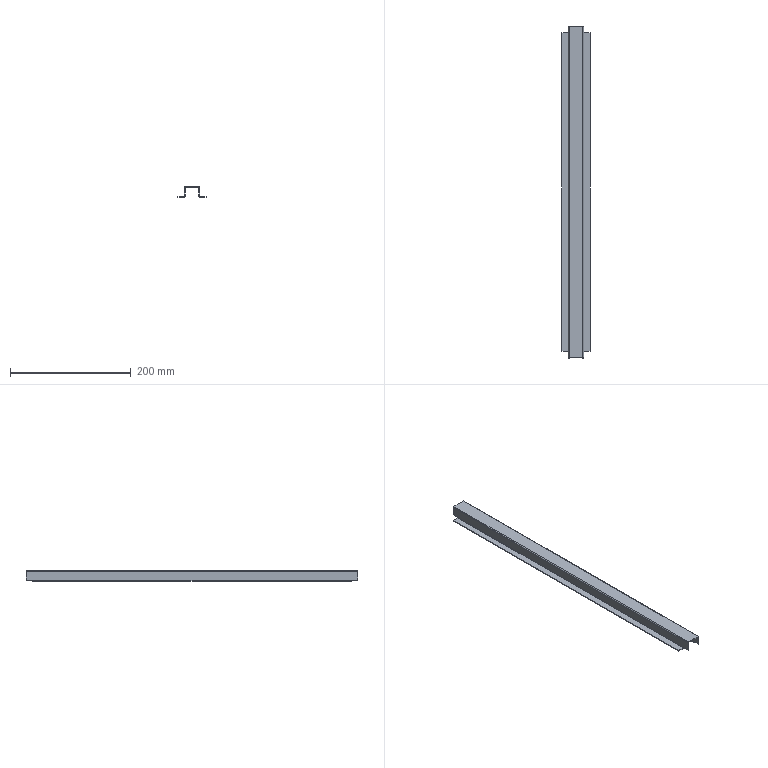Part | SolidWorks | features EdgeFlange 3, FlatPattern 1, ICE 1, SMBaseFlange 1, SheetMetal 1 | 1 solid | 46 faces | box 46.6 x 550 x 18 mm | volume 51368 mm3 | plane 38 | cylinder 8 | commonest cylinder face diameters 0.4 x4 2.8 x4
STEP:
#1=CARTESIAN_POINT('',(24.665,538.707,-16.6));
#2=VERTEX_POINT('',#1);
#3=CARTESIAN_POINT('',(24.665,10.707,-16.6));
#4=VERTEX_POINT('',#3);
#5=CARTESIAN_POINT('',(24.665,538.707,-16.6));
#6=DIRECTION('',(0.,-1.,0.));
#7=VECTOR('',#6,1000.);
#8=LINE('',#5,#7);
#9=EDGE_CURVE('',#2,#4,#8,.T.);
#10=ORIENTED_EDGE('',*,*,#9,.F.);
#11=CARTESIAN_POINT('',(24.665,538.707,-16.));
#12=VERTEX_POINT('',#11);
#13=CARTESIAN_POINT('',(24.665,538.707,0.));
#14=DIRECTION('',(0.,0.,-1.));
#15=VECTOR('',#14,1000.);
#16=LINE('',#13,#15);
#17=EDGE_CURVE('',#12,#2,#16,.T.);
#18=ORIENTED_EDGE('',*,*,#17,.F.);
#19=CARTESIAN_POINT('',(24.665,549.707,-16.));
#20=VERTEX_POINT('',#19);
#21=CARTESIAN_POINT('',(24.665,0.,-16.));
#22=DIRECTION('',(0.,-1.,0.));
#23=VECTOR('',#22,1000.);
#24=LINE('',#21,#23);
#25=EDGE_CURVE('',#20,#12,#24,.T.);
#26=ORIENTED_EDGE('',*,*,#25,.F.);
#27=CARTESIAN_POINT('',(24.665,549.707,-1.4));
#28=VERTEX_POINT('',#27);
#29=CARTESIAN_POINT('',(24.665,549.707,-18.));
#30=DIRECTION('',(0.,0.,-1.));
#31=VECTOR('',#30,1000.);
#32=LINE('',#29,#31);
#33=EDGE_CURVE('',#28,#20,#32,.T.);
#34=ORIENTED_EDGE('',*,*,#33,.F.);
#35=CARTESIAN_POINT('',(24.665,-0.2928,-1.4));
#36=VERTEX_POINT('',#35);
#37=CARTESIAN_POINT('',(24.665,0.,-1.4));
#38=DIRECTION('',(0.,-1.,0.));
#39=VECTOR('',#38,1000.);
#40=LINE('',#37,#39);
#41=EDGE_CURVE('',#28,#36,#40,.T.);
#42=ORIENTED_EDGE('',*,*,#41,.T.);
#43=CARTESIAN_POINT('',(24.665,-0.2928,-16.));
#44=VERTEX_POINT('',#43);
#45=CARTESIAN_POINT('',(24.665,-0.2928,-1.2));
#46=DIRECTION('',(0.,0.,1.));
#47=VECTOR('',#46,1000.);
#48=LINE('',#45,#47);
#49=EDGE_CURVE('',#44,#36,#48,.T.);
#50=ORIENTED_EDGE('',*,*,#49,.F.);
#51=CARTESIAN_POINT('',(24.665,10.707,-16.));
#52=VERTEX_POINT('',#51);
#53=CARTESIAN_POINT('',(24.665,0.,-16.));
#54=DIRECTION('',(0.,-1.,0.));
#55=VECTOR('',#54,1000.);
#56=LINE('',#53,#55);
#57=EDGE_CURVE('',#52,#44,#56,.T.);
#58=ORIENTED_EDGE('',*,*,#57,.F.);
#59=CARTESIAN_POINT('',(24.665,10.707,0.));
#60=DIRECTION('',(0.,0.,1.));
#61=VECTOR('',#60,1000.);
#62=LINE('',#59,#61);
#63=EDGE_CURVE('',#4,#52,#62,.T.);
#64=ORIENTED_EDGE('',*,*,#63,.F.);
#65=EDGE_LOOP('',(#10,#18,#26,#34,#42,#50,#58,#64));
#66=FACE_OUTER_BOUND('',#65,.T.);
#67=CARTESIAN_POINT('',(24.665,0.,0.));
#68=DIRECTION('',(1.,0.,0.));
#69=DIRECTION('',(0.,0.,-1.));
#70=AXIS2_PLACEMENT_3D('',#67,#68,#69);
#71=PLANE('',#70);
#72=ADVANCED_FACE('',(#66),#71,.T.);
#73=CARTESIAN_POINT('',(23.465,538.707,-16.));
#74=VERTEX_POINT('',#73);
#75=CARTESIAN_POINT('',(23.465,538.707,-16.6));
#76=VERTEX_POINT('',#75);
#77=CARTESIAN_POINT('',(23.465,538.707,0.));
#78=DIRECTION('',(0.,0.,-1.));
#79=VECTOR('',#78,1000.);
#80=LINE('',#77,#79);
#81=EDGE_CURVE('',#74,#76,#80,.T.);
#82=ORIENTED_EDGE('',*,*,#81,.T.);
#83=CARTESIAN_POINT('',(23.465,10.707,-16.6));
#84=VERTEX_POINT('',#83);
#85=CARTESIAN_POINT('',(23.465,538.707,-16.6));
#86=DIRECTION('',(0.,-1.,0.));
#87=VECTOR('',#86,1000.);
#88=LINE('',#85,#87);
#89=EDGE_CURVE('',#76,#84,#88,.T.);
#90=ORIENTED_EDGE('',*,*,#89,.T.);
#91=CARTESIAN_POINT('',(23.465,10.707,-16.));
#92=VERTEX_POINT('',#91);
#93=CARTESIAN_POINT('',(23.465,10.707,0.));
#94=DIRECTION('',(0.,0.,1.));
#95=VECTOR('',#94,1000.);
#96=LINE('',#93,#95);
#97=EDGE_CURVE('',#84,#92,#96,.T.);
#98=ORIENTED_EDGE('',*,*,#97,.T.);
#99=CARTESIAN_POINT('',(23.465,-0.2928,-16.));
#100=VERTEX_POINT('',#99);
#101=CARTESIAN_POINT('',(23.465,0.,-16.));
#102=DIRECTION('',(0.,-1.,0.));
#103=VECTOR('',#102,1000.);
#104=LINE('',#101,#103);
#105=EDGE_CURVE('',#92,#100,#104,.T.);
#106=ORIENTED_EDGE('',*,*,#105,.T.);
#107=CARTESIAN_POINT('',(23.465,-0.2928,-1.4));
#108=VERTEX_POINT('',#107);
#109=CARTESIAN_POINT('',(23.465,-0.2928,0.));
#110=DIRECTION('',(0.,0.,1.));
#111=VECTOR('',#110,1000.);
#112=LINE('',#109,#111);
#113=EDGE_CURVE('',#100,#108,#112,.T.);
#114=ORIENTED_EDGE('',*,*,#113,.T.);
#115=CARTESIAN_POINT('',(23.465,549.707,-1.4));
#116=VERTEX_POINT('',#115);
#117=CARTESIAN_POINT('',(23.465,549.707,-1.4));
#118=DIRECTION('',(0.,-1.,0.));
#119=VECTOR('',#118,1000.);
#120=LINE('',#117,#119);
#121=EDGE_CURVE('',#116,#108,#120,.T.);
#122=ORIENTED_EDGE('',*,*,#121,.F.);
#123=CARTESIAN_POINT('',(23.465,549.707,-16.));
#124=VERTEX_POINT('',#123);
#125=CARTESIAN_POINT('',(23.465,549.707,0.));
#126=DIRECTION('',(0.,0.,-1.));
#127=VECTOR('',#126,1000.);
#128=LINE('',#125,#127);
#129=EDGE_CURVE('',#116,#124,#128,.T.);
#130=ORIENTED_EDGE('',*,*,#129,.T.);
#131=CARTESIAN_POINT('',(23.465,0.,-16.));
#132=DIRECTION('',(0.,-1.,0.));
#133=VECTOR('',#132,1000.);
#134=LINE('',#131,#133);
#135=EDGE_CURVE('',#124,#74,#134,.T.);
#136=ORIENTED_EDGE('',*,*,#135,.T.);
#137=EDGE_LOOP('',(#82,#90,#98,#106,#114,#122,#130,#136));
#138=FACE_OUTER_BOUND('',#137,.T.);
#139=CARTESIAN_POINT('',(23.465,0.,0.));
#140=DIRECTION('',(1.,0.,0.));
#141=DIRECTION('',(0.,0.,-1.));
#142=AXIS2_PLACEMENT_3D('',#139,#140,#141);
#143=PLANE('',#142);
#144=ADVANCED_FACE('',(#138),#143,.F.);
#145=ORIENTED_EDGE('',*,*,#33,.T.);
#146=CARTESIAN_POINT('',(23.465,549.707,-16.));
#147=DIRECTION('',(1.,0.,0.));
#148=VECTOR('',#147,1000.);
#149=LINE('',#146,#148);
#150=EDGE_CURVE('',#124,#20,#149,.T.);
#151=ORIENTED_EDGE('',*,*,#150,.F.);
#152=ORIENTED_EDGE('',*,*,#129,.F.);
#153=CARTESIAN_POINT('',(24.665,549.707,-1.4));
#154=DIRECTION('',(1.,0.,0.));
#155=VECTOR('',#154,1000.);
#156=LINE('',#153,#155);
#157=EDGE_CURVE('',#116,#28,#156,.T.);
#158=ORIENTED_EDGE('',*,*,#157,.T.);
#159=EDGE_LOOP('',(#145,#151,#152,#158));
#160=FACE_OUTER_BOUND('',#159,.T.);
#161=CARTESIAN_POINT('',(24.665,549.707,-18.));
#162=DIRECTION('',(0.,1.,0.));
#163=DIRECTION('',(0.,0.,1.));
#164=AXIS2_PLACEMENT_3D('',#161,#162,#163);
#165=PLANE('',#164);
#166=ADVANCED_FACE('',(#160),#165,.T.);
#167=CARTESIAN_POINT('',(-0.3354,10.707,-16.));
#168=VERTEX_POINT('',#167);
#169=CARTESIAN_POINT('',(-0.3354,-0.2928,-16.));
#170=VERTEX_POINT('',#169);
#171=CARTESIAN_POINT('',(-0.3354,0.,-16.));
#172=DIRECTION('',(0.,-1.,0.));
#173=VECTOR('',#172,1000.);
#174=LINE('',#171,#173);
#175=EDGE_CURVE('',#168,#170,#174,.T.);
#176=ORIENTED_EDGE('',*,*,#175,.T.);
#177=CARTESIAN_POINT('',(-0.3354,-0.2928,-1.4));
#178=VERTEX_POINT('',#177);
#179=CARTESIAN_POINT('',(-0.3354,-0.2928,-1.2));
#180=DIRECTION('',(0.,0.,-1.));
#181=VECTOR('',#180,1000.);
#182=LINE('',#179,#181);
#183=EDGE_CURVE('',#178,#170,#182,.T.);
#184=ORIENTED_EDGE('',*,*,#183,.F.);
#185=CARTESIAN_POINT('',(-0.3354,549.707,-1.4));
#186=VERTEX_POINT('',#185);
#187=CARTESIAN_POINT('',(-0.3354,-0.2928,-1.4));
#188=DIRECTION('',(0.,-1.,0.));
#189=VECTOR('',#188,1000.);
#190=LINE('',#187,#189);
#191=EDGE_CURVE('',#186,#178,#190,.T.);
#192=ORIENTED_EDGE('',*,*,#191,.F.);
#193=CARTESIAN_POINT('',(-0.3354,549.707,-16.));
#194=VERTEX_POINT('',#193);
#195=CARTESIAN_POINT('',(-0.3354,549.707,-18.));
#196=DIRECTION('',(0.,0.,1.));
#197=VECTOR('',#196,1000.);
#198=LINE('',#195,#197);
#199=EDGE_CURVE('',#194,#186,#198,.T.);
#200=ORIENTED_EDGE('',*,*,#199,.F.);
#201=CARTESIAN_POINT('',(-0.3354,538.707,-16.));
#202=VERTEX_POINT('',#201);
#203=CARTESIAN_POINT('',(-0.3354,0.,-16.));
#204=DIRECTION('',(0.,-1.,0.));
#205=VECTOR('',#204,1000.);
#206=LINE('',#203,#205);
#207=EDGE_CURVE('',#194,#202,#206,.T.);
#208=ORIENTED_EDGE('',*,*,#207,.T.);
#209=CARTESIAN_POINT('',(-0.3354,538.707,-16.6));
#210=VERTEX_POINT('',#209);
#211=CARTESIAN_POINT('',(-0.3354,538.707,0.));
#212=DIRECTION('',(0.,0.,-1.));
#213=VECTOR('',#212,1000.);
#214=LINE('',#211,#213);
#215=EDGE_CURVE('',#202,#210,#214,.T.);
#216=ORIENTED_EDGE('',*,*,#215,.T.);
#217=CARTESIAN_POINT('',(-0.3354,10.707,-16.6));
#218=VERTEX_POINT('',#217);
#219=CARTESIAN_POINT('',(-0.3354,10.707,-16.6));
#220=DIRECTION('',(0.,1.,0.));
#221=VECTOR('',#220,1000.);
#222=LINE('',#219,#221);
#223=EDGE_CURVE('',#218,#210,#222,.T.);
#224=ORIENTED_EDGE('',*,*,#223,.F.);
#225=CARTESIAN_POINT('',(-0.3354,10.707,0.));
#226=DIRECTION('',(0.,0.,1.));
#227=VECTOR('',#226,1000.);
#228=LINE('',#225,#227);
#229=EDGE_CURVE('',#218,#168,#228,.T.);
#230=ORIENTED_EDGE('',*,*,#229,.T.);
#231=EDGE_LOOP('',(#176,#184,#192,#200,#208,#216,#224,#230));
#232=FACE_OUTER_BOUND('',#231,.T.);
#233=CARTESIAN_POINT('',(-0.3354,0.,0.));
#234=DIRECTION('',(1.,0.,0.));
#235=DIRECTION('',(0.,0.,-1.));
#236=AXIS2_PLACEMENT_3D('',#233,#234,#235);
#237=PLANE('',#236);
#238=ADVANCED_FACE('',(#232),#237,.F.);
#239=CARTESIAN_POINT('',(0.8646,-0.2928,-1.4));
#240=VERTEX_POINT('',#239);
#241=CARTESIAN_POINT('',(0.8646,-0.2928,-16.));
#242=VERTEX_POINT('',#241);
#243=CARTESIAN_POINT('',(0.8646,-0.2928,0.));
#244=DIRECTION('',(0.,0.,-1.));
#245=VECTOR('',#244,1000.);
#246=LINE('',#243,#245);
#247=EDGE_CURVE('',#240,#242,#246,.T.);
#248=ORIENTED_EDGE('',*,*,#247,.T.);
#249=CARTESIAN_POINT('',(0.8646,10.707,-16.));
#250=VERTEX_POINT('',#249);
#251=CARTESIAN_POINT('',(0.8646,0.,-16.));
#252=DIRECTION('',(0.,-1.,0.));
#253=VECTOR('',#252,1000.);
#254=LINE('',#251,#253);
#255=EDGE_CURVE('',#250,#242,#254,.T.);
#256=ORIENTED_EDGE('',*,*,#255,.F.);
#257=CARTESIAN_POINT('',(0.8646,10.707,-16.6));
#258=VERTEX_POINT('',#257);
#259=CARTESIAN_POINT('',(0.8646,10.707,0.));
#260=DIRECTION('',(0.,0.,1.));
#261=VECTOR('',#260,1000.);
#262=LINE('',#259,#261);
#263=EDGE_CURVE('',#258,#250,#262,.T.);
#264=ORIENTED_EDGE('',*,*,#263,.F.);
#265=CARTESIAN_POINT('',(0.8646,538.707,-16.6));
#266=VERTEX_POINT('',#265);
#267=CARTESIAN_POINT('',(0.8646,10.707,-16.6));
#268=DIRECTION('',(0.,1.,0.));
#269=VECTOR('',#268,1000.);
#270=LINE('',#267,#269);
#271=EDGE_CURVE('',#258,#266,#270,.T.);
#272=ORIENTED_EDGE('',*,*,#271,.T.);
#273=CARTESIAN_POINT('',(0.8646,538.707,-16.));
#274=VERTEX_POINT('',#273);
#275=CARTESIAN_POINT('',(0.8646,538.707,0.));
#276=DIRECTION('',(0.,0.,-1.));
#277=VECTOR('',#276,1000.);
#278=LINE('',#275,#277);
#279=EDGE_CURVE('',#274,#266,#278,.T.);
#280=ORIENTED_EDGE('',*,*,#279,.F.);
#281=CARTESIAN_POINT('',(0.8646,549.707,-16.));
#282=VERTEX_POINT('',#281);
#283=CARTESIAN_POINT('',(0.8646,0.,-16.));
#284=DIRECTION('',(0.,-1.,0.));
#285=VECTOR('',#284,1000.);
#286=LINE('',#283,#285);
#287=EDGE_CURVE('',#282,#274,#286,.T.);
#288=ORIENTED_EDGE('',*,*,#287,.F.);
#289=CARTESIAN_POINT('',(0.8646,549.707,-1.4));
#290=VERTEX_POINT('',#289);
#291=CARTESIAN_POINT('',(0.8646,549.707,0.));
#292=DIRECTION('',(0.,0.,1.));
#293=VECTOR('',#292,1000.);
#294=LINE('',#291,#293);
#295=EDGE_CURVE('',#282,#290,#294,.T.);
#296=ORIENTED_EDGE('',*,*,#295,.T.);
#297=CARTESIAN_POINT('',(0.8646,-0.2928,-1.4));
#298=DIRECTION('',(0.,1.,0.));
#299=VECTOR('',#298,1000.);
#300=LINE('',#297,#299);
#301=EDGE_CURVE('',#240,#290,#300,.T.);
#302=ORIENTED_EDGE('',*,*,#301,.F.);
#303=EDGE_LOOP('',(#248,#256,#264,#272,#280,#288,#296,#302));
#304=FACE_OUTER_BOUND('',#303,.T.);
#305=CARTESIAN_POINT('',(0.8646,0.,0.));
#306=DIRECTION('',(1.,0.,0.));
#307=DIRECTION('',(0.,0.,-1.));
#308=AXIS2_PLACEMENT_3D('',#305,#306,#307);
#309=PLANE('',#308);
#310=ADVANCED_FACE('',(#304),#309,.T.);
#311=ORIENTED_EDGE('',*,*,#183,.T.);
#312=CARTESIAN_POINT('',(-0.3354,-0.2928,-16.));
#313=DIRECTION('',(1.,0.,0.));
#314=VECTOR('',#313,1000.);
#315=LINE('',#312,#314);
#316=EDGE_CURVE('',#170,#242,#315,.T.);
#317=ORIENTED_EDGE('',*,*,#316,.T.);
#318=ORIENTED_EDGE('',*,*,#247,.F.);
#319=CARTESIAN_POINT('',(-0.3354,-0.2928,-1.4));
#320=DIRECTION('',(-1.,0.,0.));
#321=VECTOR('',#320,1000.);
#322=LINE('',#319,#321);
#323=EDGE_CURVE('',#240,#178,#322,.T.);
#324=ORIENTED_EDGE('',*,*,#323,.T.);
#325=EDGE_LOOP('',(#311,#317,#318,#324));
#326=FACE_OUTER_BOUND('',#325,.T.);
#327=CARTESIAN_POINT('',(-0.3354,-0.2928,-1.2));
#328=DIRECTION('',(0.,-1.,0.));
#329=DIRECTION('',(0.,0.,-1.));
#330=AXIS2_PLACEMENT_3D('',#327,#328,#329);
#331=PLANE('',#330);
#332=ADVANCED_FACE('',(#326),#331,.T.);
#333=ORIENTED_EDGE('',*,*,#295,.F.);
#334=CARTESIAN_POINT('',(-0.3354,549.707,-16.));
#335=DIRECTION('',(1.,0.,0.));
#336=VECTOR('',#335,1000.);
#337=LINE('',#334,#336);
#338=EDGE_CURVE('',#194,#282,#337,.T.);
#339=ORIENTED_EDGE('',*,*,#338,.F.);
#340=ORIENTED_EDGE('',*,*,#199,.T.);
#341=CARTESIAN_POINT('',(0.8646,549.707,-1.4));
#342=DIRECTION('',(-1.,0.,0.));
#343=VECTOR('',#342,1000.);
#344=LINE('',#341,#343);
#345=EDGE_CURVE('',#290,#186,#344,.T.);
#346=ORIENTED_EDGE('',*,*,#345,.F.);
#347=EDGE_LOOP('',(#333,#339,#340,#346));
#348=FACE_OUTER_BOUND('',#347,.T.);
#349=CARTESIAN_POINT('',(-0.3354,549.707,-18.));
#350=DIRECTION('',(0.,1.,0.));
#351=DIRECTION('',(0.,0.,1.));
#352=AXIS2_PLACEMENT_3D('',#349,#350,#351);
#353=PLANE('',#352);
#354=ADVANCED_FACE('',(#348),#353,.T.);
#355=ORIENTED_EDGE('',*,*,#113,.F.);
#356=CARTESIAN_POINT('',(23.465,-0.2928,-16.));
#357=DIRECTION('',(1.,0.,0.));
#358=VECTOR('',#357,1000.);
#359=LINE('',#356,#358);
#360=EDGE_CURVE('',#100,#44,#359,.T.);
#361=ORIENTED_EDGE('',*,*,#360,.T.);
#362=ORIENTED_EDGE('',*,*,#49,.T.);
#363=CARTESIAN_POINT('',(23.465,-0.2928,-1.4));
#364=DIRECTION('',(1.,0.,0.));
#365=VECTOR('',#364,1000.);
#366=LINE('',#363,#365);
#367=EDGE_CURVE('',#108,#36,#366,.T.);
#368=ORIENTED_EDGE('',*,*,#367,.F.);
#369=EDGE_LOOP('',(#355,#361,#362,#368));
#370=FACE_OUTER_BOUND('',#369,.T.);
#371=CARTESIAN_POINT('',(24.665,-0.2928,-1.2));
#372=DIRECTION('',(0.,-1.,0.));
#373=DIRECTION('',(0.,0.,-1.));
#374=AXIS2_PLACEMENT_3D('',#371,#372,#373);
#375=PLANE('',#374);
#376=ADVANCED_FACE('',(#370),#375,.T.);
#377=CARTESIAN_POINT('',(1.065,-0.2928,-1.2));
#378=VERTEX_POINT('',#377);
#379=CARTESIAN_POINT('',(23.265,-0.2928,-1.2));
#380=VERTEX_POINT('',#379);
#381=CARTESIAN_POINT('',(-0.3354,-0.2928,-1.2));
#382=DIRECTION('',(1.,0.,0.));
#383=VECTOR('',#382,1000.);
#384=LINE('',#381,#383);
#385=EDGE_CURVE('',#378,#380,#384,.T.);
#386=ORIENTED_EDGE('',*,*,#385,.F.);
#387=CARTESIAN_POINT('',(1.065,549.707,-1.2));
#388=VERTEX_POINT('',#387);
#389=CARTESIAN_POINT('',(1.065,549.707,-1.2));
#390=DIRECTION('',(0.,-1.,0.));
#391=VECTOR('',#390,1000.);
#392=LINE('',#389,#391);
#393=EDGE_CURVE('',#388,#378,#392,.T.);
#394=ORIENTED_EDGE('',*,*,#393,.F.);
#395=CARTESIAN_POINT('',(23.265,549.707,-1.2));
#396=VERTEX_POINT('',#395);
#397=CARTESIAN_POINT('',(-0.3354,549.707,-1.2));
#398=DIRECTION('',(-1.,0.,0.));
#399=VECTOR('',#398,1000.);
#400=LINE('',#397,#399);
#401=EDGE_CURVE('',#396,#388,#400,.T.);
#402=ORIENTED_EDGE('',*,*,#401,.F.);
#403=CARTESIAN_POINT('',(23.265,-0.2928,-1.2));
#404=DIRECTION('',(0.,1.,0.));
#405=VECTOR('',#404,1000.);
#406=LINE('',#403,#405);
#407=EDGE_CURVE('',#380,#396,#406,.T.);
#408=ORIENTED_EDGE('',*,*,#407,.F.);
#409=EDGE_LOOP('',(#386,#394,#402,#408));
#410=FACE_OUTER_BOUND('',#409,.T.);
#411=CARTESIAN_POINT('',(0.,0.,-1.2));
#412=DIRECTION('',(0.,0.,-1.));
#413=DIRECTION('',(-1.,0.,0.));
#414=AXIS2_PLACEMENT_3D('',#411,#412,#413);
#415=PLANE('',#414);
#416=ADVANCED_FACE('',(#410),#415,.T.);
#417=CARTESIAN_POINT('',(1.065,549.707,0.));
#418=VERTEX_POINT('',#417);
#419=CARTESIAN_POINT('',(1.065,-0.2928,0.));
#420=VERTEX_POINT('',#419);
#421=CARTESIAN_POINT('',(1.065,549.707,0.));
#422=DIRECTION('',(0.,-1.,0.));
#423=VECTOR('',#422,1000.);
#424=LINE('',#421,#423);
#425=EDGE_CURVE('',#418,#420,#424,.T.);
#426=ORIENTED_EDGE('',*,*,#425,.T.);
#427=CARTESIAN_POINT('',(23.265,-0.2928,0.));
#428=VERTEX_POINT('',#427);
#429=CARTESIAN_POINT('',(-0.3354,-0.2928,0.));
#430=DIRECTION('',(1.,0.,0.));
#431=VECTOR('',#430,1000.);
#432=LINE('',#429,#431);
#433=EDGE_CURVE('',#420,#428,#432,.T.);
#434=ORIENTED_EDGE('',*,*,#433,.T.);
#435=CARTESIAN_POINT('',(23.265,549.707,0.));
#436=VERTEX_POINT('',#435);
#437=CARTESIAN_POINT('',(23.265,-0.2928,0.));
#438=DIRECTION('',(0.,1.,0.));
#439=VECTOR('',#438,1000.);
#440=LINE('',#437,#439);
#441=EDGE_CURVE('',#428,#436,#440,.T.);
#442=ORIENTED_EDGE('',*,*,#441,.T.);
#443=CARTESIAN_POINT('',(-0.3354,549.707,0.));
#444=DIRECTION('',(-1.,0.,0.));
#445=VECTOR('',#444,1000.);
#446=LINE('',#443,#445);
#447=EDGE_CURVE('',#436,#418,#446,.T.);
#448=ORIENTED_EDGE('',*,*,#447,.T.);
#449=EDGE_LOOP('',(#426,#434,#442,#448));
#450=FACE_OUTER_BOUND('',#449,.T.);
#451=CARTESIAN_POINT('',(0.,0.,0.));
#452=DIRECTION('',(0.,0.,-1.));
#453=DIRECTION('',(-1.,0.,0.));
#454=AXIS2_PLACEMENT_3D('',#451,#452,#453);
#455=PLANE('',#454);
#456=ADVANCED_FACE('',(#450),#455,.F.);
#457=ORIENTED_EDGE('',*,*,#401,.T.);
#458=CARTESIAN_POINT('',(1.065,549.707,-1.2));
#459=DIRECTION('',(0.,0.,1.));
#460=VECTOR('',#459,1000.);
#461=LINE('',#458,#460);
#462=EDGE_CURVE('',#388,#418,#461,.T.);
#463=ORIENTED_EDGE('',*,*,#462,.T.);
#464=ORIENTED_EDGE('',*,*,#447,.F.);
#465=CARTESIAN_POINT('',(23.265,549.707,-1.2));
#466=DIRECTION('',(0.,0.,1.));
#467=VECTOR('',#466,1000.);
#468=LINE('',#465,#467);
#469=EDGE_CURVE('',#396,#436,#468,.T.);
#470=ORIENTED_EDGE('',*,*,#469,.F.);
#471=EDGE_LOOP('',(#457,#463,#464,#470));
#472=FACE_OUTER_BOUND('',#471,.T.);
#473=CARTESIAN_POINT('',(-0.3354,549.707,-1.2));
#474=DIRECTION('',(0.,1.,0.));
#475=DIRECTION('',(0.,0.,1.));
#476=AXIS2_PLACEMENT_3D('',#473,#474,#475);
#477=PLANE('',#476);
#478=ADVANCED_FACE('',(#472),#477,.T.);
#479=CARTESIAN_POINT('',(1.065,-0.2928,-1.2));
#480=DIRECTION('',(0.,0.,1.));
#481=VECTOR('',#480,1000.);
#482=LINE('',#479,#481);
#483=EDGE_CURVE('',#378,#420,#482,.T.);
#484=ORIENTED_EDGE('',*,*,#483,.F.);
#485=ORIENTED_EDGE('',*,*,#385,.T.);
#486=CARTESIAN_POINT('',(23.265,-0.2928,-1.2));
#487=DIRECTION('',(0.,0.,1.));
#488=VECTOR('',#487,1000.);
#489=LINE('',#486,#488);
#490=EDGE_CURVE('',#380,#428,#489,.T.);
#491=ORIENTED_EDGE('',*,*,#490,.T.);
#492=ORIENTED_EDGE('',*,*,#433,.F.);
#493=EDGE_LOOP('',(#484,#485,#491,#492));
#494=FACE_OUTER_BOUND('',#493,.T.);
#495=CARTESIAN_POINT('',(-0.3354,-0.2928,-1.2));
#496=DIRECTION('',(0.,-1.,0.));
#497=DIRECTION('',(0.,0.,-1.));
#498=AXIS2_PLACEMENT_3D('',#495,#496,#497);
#499=PLANE('',#498);
#500=ADVANCED_FACE('',(#494),#499,.T.);
#501=ORIENTED_EDGE('',*,*,#157,.F.);
#502=CARTESIAN_POINT('',(23.265,549.707,-1.4));
#503=DIRECTION('',(0.,1.,0.));
#504=DIRECTION('',(0.,0.,-1.));
#505=AXIS2_PLACEMENT_3D('',#502,#503,#504);
#506=CIRCLE('',#505,0.2);
#507=EDGE_CURVE('',#396,#116,#506,.T.);
#508=ORIENTED_EDGE('',*,*,#507,.F.);
#509=ORIENTED_EDGE('',*,*,#469,.T.);
#510=CARTESIAN_POINT('',(23.265,549.707,-1.4));
#511=DIRECTION('',(0.,1.,0.));
#512=DIRECTION('',(0.,0.,-1.));
#513=AXIS2_PLACEMENT_3D('',#510,#511,#512);
#514=CIRCLE('',#513,1.4);
#515=EDGE_CURVE('',#436,#28,#514,.T.);
#516=ORIENTED_EDGE('',*,*,#515,.T.);
#517=EDGE_LOOP('',(#501,#508,#509,#516));
#518=FACE_OUTER_BOUND('',#517,.T.);
#519=CARTESIAN_POINT('',(23.265,549.707,-1.4));
#520=DIRECTION('',(0.,1.,0.));
#521=DIRECTION('',(0.,0.,1.));
#522=AXIS2_PLACEMENT_3D('',#519,#520,#521);
#523=PLANE('',#522);
#524=ADVANCED_FACE('',(#518),#523,.T.);
#525=CARTESIAN_POINT('',(23.265,-0.2928,-1.4));
#526=DIRECTION('',(0.,-1.,0.));
#527=DIRECTION('',(0.,0.,-1.));
#528=AXIS2_PLACEMENT_3D('',#525,#526,#527);
#529=CIRCLE('',#528,0.2);
#530=EDGE_CURVE('',#108,#380,#529,.T.);
#531=ORIENTED_EDGE('',*,*,#530,.F.);
#532=ORIENTED_EDGE('',*,*,#367,.T.);
#533=CARTESIAN_POINT('',(23.265,-0.2928,-1.4));
#534=DIRECTION('',(0.,-1.,0.));
#535=DIRECTION('',(0.,0.,-1.));
#536=AXIS2_PLACEMENT_3D('',#533,#534,#535);
#537=CIRCLE('',#536,1.4);
#538=EDGE_CURVE('',#36,#428,#537,.T.);
#539=ORIENTED_EDGE('',*,*,#538,.T.);
#540=ORIENTED_EDGE('',*,*,#490,.F.);
#541=EDGE_LOOP('',(#531,#532,#539,#540));
#542=FACE_OUTER_BOUND('',#541,.T.);
#543=CARTESIAN_POINT('',(23.265,-0.2928,-1.4));
#544=DIRECTION('',(0.,1.,0.));
#545=DIRECTION('',(0.,0.,1.));
#546=AXIS2_PLACEMENT_3D('',#543,#544,#545);
#547=PLANE('',#546);
#548=ADVANCED_FACE('',(#542),#547,.F.);
#549=ORIENTED_EDGE('',*,*,#441,.F.);
#550=ORIENTED_EDGE('',*,*,#538,.F.);
#551=ORIENTED_EDGE('',*,*,#41,.F.);
#552=ORIENTED_EDGE('',*,*,#515,.F.);
#553=EDGE_LOOP('',(#549,#550,#551,#552));
#554=FACE_OUTER_BOUND('',#553,.T.);
#555=CARTESIAN_POINT('',(23.265,-0.2928,-1.4));
#556=DIRECTION('',(0.,-1.,0.));
#557=DIRECTION('',(1.,0.,0.));
#558=AXIS2_PLACEMENT_3D('',#555,#556,#557);
#559=CYLINDRICAL_SURFACE('',#558,1.4);
#560=ADVANCED_FACE('',(#554),#559,.T.);
#561=ORIENTED_EDGE('',*,*,#407,.T.);
#562=ORIENTED_EDGE('',*,*,#507,.T.);
#563=ORIENTED_EDGE('',*,*,#121,.T.);
#564=ORIENTED_EDGE('',*,*,#530,.T.);
#565=EDGE_LOOP('',(#561,#562,#563,#564));
#566=FACE_OUTER_BOUND('',#565,.T.);
#567=CARTESIAN_POINT('',(23.265,-0.2928,-1.4));
#568=DIRECTION('',(0.,-1.,0.));
#569=DIRECTION('',(1.,0.,0.));
#570=AXIS2_PLACEMENT_3D('',#567,#568,#569);
#571=CYLINDRICAL_SURFACE('',#570,0.2);
#572=ADVANCED_FACE('',(#566),#571,.F.);
#573=ORIENTED_EDGE('',*,*,#323,.F.);
#574=CARTESIAN_POINT('',(1.065,-0.2928,-1.4));
#575=DIRECTION('',(0.,-1.,0.));
#576=DIRECTION('',(0.,0.,1.));
#577=AXIS2_PLACEMENT_3D('',#574,#575,#576);
#578=CIRCLE('',#577,0.2);
#579=EDGE_CURVE('',#378,#240,#578,.T.);
#580=ORIENTED_EDGE('',*,*,#579,.F.);
#581=ORIENTED_EDGE('',*,*,#483,.T.);
#582=CARTESIAN_POINT('',(1.065,-0.2928,-1.4));
#583=DIRECTION('',(0.,-1.,0.));
#584=DIRECTION('',(0.,0.,1.));
#585=AXIS2_PLACEMENT_3D('',#582,#583,#584);
#586=CIRCLE('',#585,1.4);
#587=EDGE_CURVE('',#420,#178,#586,.T.);
#588=ORIENTED_EDGE('',*,*,#587,.T.);
#589=EDGE_LOOP('',(#573,#580,#581,#588));
#590=FACE_OUTER_BOUND('',#589,.T.);
#591=CARTESIAN_POINT('',(1.065,-0.2928,-1.4));
#592=DIRECTION('',(0.,-1.,0.));
#593=DIRECTION('',(0.,0.,-1.));
#594=AXIS2_PLACEMENT_3D('',#591,#592,#593);
#595=PLANE('',#594);
#596=ADVANCED_FACE('',(#590),#595,.T.);
#597=CARTESIAN_POINT('',(1.065,549.707,-1.4));
#598=DIRECTION('',(0.,1.,0.));
#599=DIRECTION('',(0.,0.,1.));
#600=AXIS2_PLACEMENT_3D('',#597,#598,#599);
#601=CIRCLE('',#600,0.2);
#602=EDGE_CURVE('',#290,#388,#601,.T.);
#603=ORIENTED_EDGE('',*,*,#602,.F.);
#604=ORIENTED_EDGE('',*,*,#345,.T.);
#605=CARTESIAN_POINT('',(1.065,549.707,-1.4));
#606=DIRECTION('',(0.,1.,0.));
#607=DIRECTION('',(0.,0.,1.));
#608=AXIS2_PLACEMENT_3D('',#605,#606,#607);
#609=CIRCLE('',#608,1.4);
#610=EDGE_CURVE('',#186,#418,#609,.T.);
#611=ORIENTED_EDGE('',*,*,#610,.T.);
#612=ORIENTED_EDGE('',*,*,#462,.F.);
#613=EDGE_LOOP('',(#603,#604,#611,#612));
#614=FACE_OUTER_BOUND('',#613,.T.);
#615=CARTESIAN_POINT('',(1.065,549.707,-1.4));
#616=DIRECTION('',(0.,-1.,0.));
#617=DIRECTION('',(0.,0.,-1.));
#618=AXIS2_PLACEMENT_3D('',#615,#616,#617);
#619=PLANE('',#618);
#620=ADVANCED_FACE('',(#614),#619,.F.);
#621=ORIENTED_EDGE('',*,*,#425,.F.);
#622=ORIENTED_EDGE('',*,*,#610,.F.);
#623=ORIENTED_EDGE('',*,*,#191,.T.);
#624=ORIENTED_EDGE('',*,*,#587,.F.);
#625=EDGE_LOOP('',(#621,#622,#623,#624));
#626=FACE_OUTER_BOUND('',#625,.T.);
#627=CARTESIAN_POINT('',(1.065,549.707,-1.4));
#628=DIRECTION('',(0.,1.,0.));
#629=DIRECTION('',(-1.,0.,0.));
#630=AXIS2_PLACEMENT_3D('',#627,#628,#629);
#631=CYLINDRICAL_SURFACE('',#630,1.4);
#632=ADVANCED_FACE('',(#626),#631,.T.);
#633=ORIENTED_EDGE('',*,*,#393,.T.);
#634=ORIENTED_EDGE('',*,*,#579,.T.);
#635=ORIENTED_EDGE('',*,*,#301,.T.);
#636=ORIENTED_EDGE('',*,*,#602,.T.);
#637=EDGE_LOOP('',(#633,#634,#635,#636));
#638=FACE_OUTER_BOUND('',#637,.T.);
#639=CARTESIAN_POINT('',(1.065,549.707,-1.4));
#640=DIRECTION('',(0.,1.,0.));
#641=DIRECTION('',(-1.,0.,0.));
#642=AXIS2_PLACEMENT_3D('',#639,#640,#641);
#643=CYLINDRICAL_SURFACE('',#642,0.2);
#644=ADVANCED_FACE('',(#638),#643,.F.);
#645=CARTESIAN_POINT('',(24.865,10.707,-16.8));
#646=VERTEX_POINT('',#645);
#647=CARTESIAN_POINT('',(24.865,10.707,-16.6));
#648=DIRECTION('',(0.,-1.,0.));
#649=DIRECTION('',(0.,0.,1.));
#650=AXIS2_PLACEMENT_3D('',#647,#648,#649);
#651=CIRCLE('',#650,0.2);
#652=EDGE_CURVE('',#4,#646,#651,.T.);
#653=ORIENTED_EDGE('',*,*,#652,.F.);
#654=CARTESIAN_POINT('',(23.465,10.707,-16.6));
#655=DIRECTION('',(1.,0.,0.));
#656=VECTOR('',#655,1000.);
#657=LINE('',#654,#656);
#658=EDGE_CURVE('',#84,#4,#657,.T.);
#659=ORIENTED_EDGE('',*,*,#658,.F.);
#660=CARTESIAN_POINT('',(24.865,10.707,-18.));
#661=VERTEX_POINT('',#660);
#662=CARTESIAN_POINT('',(24.865,10.707,-16.6));
#663=DIRECTION('',(0.,-1.,0.));
#664=DIRECTION('',(0.,0.,1.));
#665=AXIS2_PLACEMENT_3D('',#662,#663,#664);
#666=CIRCLE('',#665,1.4);
#667=EDGE_CURVE('',#84,#661,#666,.T.);
#668=ORIENTED_EDGE('',*,*,#667,.T.);
#669=CARTESIAN_POINT('',(24.865,10.707,-18.));
#670=DIRECTION('',(0.,0.,-1.));
#671=VECTOR('',#670,1000.);
#672=LINE('',#669,#671);
#673=EDGE_CURVE('',#646,#661,#672,.T.);
#674=ORIENTED_EDGE('',*,*,#673,.F.);
#675=EDGE_LOOP('',(#653,#659,#668,#674));
#676=FACE_OUTER_BOUND('',#675,.T.);
#677=CARTESIAN_POINT('',(24.865,10.707,-16.6));
#678=DIRECTION('',(0.,-1.,0.));
#679=DIRECTION('',(0.,0.,-1.));
#680=AXIS2_PLACEMENT_3D('',#677,#678,#679);
#681=PLANE('',#680);
#682=ADVANCED_FACE('',(#676),#681,.T.);
#683=CARTESIAN_POINT('',(24.865,538.707,-16.8));
#684=VERTEX_POINT('',#683);
#685=CARTESIAN_POINT('',(24.865,538.707,-18.));
#686=VERTEX_POINT('',#685);
#687=CARTESIAN_POINT('',(24.865,538.707,-16.8));
#688=DIRECTION('',(0.,0.,-1.));
#689=VECTOR('',#688,1000.);
#690=LINE('',#687,#689);
#691=EDGE_CURVE('',#684,#686,#690,.T.);
#692=ORIENTED_EDGE('',*,*,#691,.T.);
#693=CARTESIAN_POINT('',(24.865,538.707,-16.6));
#694=DIRECTION('',(0.,1.,0.));
#695=DIRECTION('',(0.,0.,1.));
#696=AXIS2_PLACEMENT_3D('',#693,#694,#695);
#697=CIRCLE('',#696,1.4);
#698=EDGE_CURVE('',#686,#76,#697,.T.);
#699=ORIENTED_EDGE('',*,*,#698,.T.);
#700=CARTESIAN_POINT('',(23.465,538.707,-16.6));
#701=DIRECTION('',(1.,0.,0.));
#702=VECTOR('',#701,1000.);
#703=LINE('',#700,#702);
#704=EDGE_CURVE('',#76,#2,#703,.T.);
#705=ORIENTED_EDGE('',*,*,#704,.T.);
#706=CARTESIAN_POINT('',(24.865,538.707,-16.6));
#707=DIRECTION('',(0.,1.,0.));
#708=DIRECTION('',(0.,0.,1.));
#709=AXIS2_PLACEMENT_3D('',#706,#707,#708);
#710=CIRCLE('',#709,0.2);
#711=EDGE_CURVE('',#684,#2,#710,.T.);
#712=ORIENTED_EDGE('',*,*,#711,.F.);
#713=EDGE_LOOP('',(#692,#699,#705,#712));
#714=FACE_OUTER_BOUND('',#713,.T.);
#715=CARTESIAN_POINT('',(24.865,538.707,-16.6));
#716=DIRECTION('',(0.,-1.,0.));
#717=DIRECTION('',(0.,0.,-1.));
#718=AXIS2_PLACEMENT_3D('',#715,#716,#717);
#719=PLANE('',#718);
#720=ADVANCED_FACE('',(#714),#719,.F.);
#721=ORIENTED_EDGE('',*,*,#89,.F.);
#722=ORIENTED_EDGE('',*,*,#698,.F.);
#723=CARTESIAN_POINT('',(24.865,0.,-18.));
#724=DIRECTION('',(0.,1.,0.));
#725=VECTOR('',#724,1000.);
#726=LINE('',#723,#725);
#727=EDGE_CURVE('',#661,#686,#726,.T.);
#728=ORIENTED_EDGE('',*,*,#727,.F.);
#729=ORIENTED_EDGE('',*,*,#667,.F.);
#730=EDGE_LOOP('',(#721,#722,#728,#729));
#731=FACE_OUTER_BOUND('',#730,.T.);
#732=CARTESIAN_POINT('',(24.865,538.707,-16.6));
#733=DIRECTION('',(0.,1.,0.));
#734=DIRECTION('',(0.,0.,-1.));
#735=AXIS2_PLACEMENT_3D('',#732,#733,#734);
#736=CYLINDRICAL_SURFACE('',#735,1.4);
#737=ADVANCED_FACE('',(#731),#736,.T.);
#738=ORIENTED_EDGE('',*,*,#9,.T.);
#739=ORIENTED_EDGE('',*,*,#652,.T.);
#740=CARTESIAN_POINT('',(24.865,10.707,-16.8));
#741=DIRECTION('',(0.,1.,0.));
#742=VECTOR('',#741,1000.);
#743=LINE('',#740,#742);
#744=EDGE_CURVE('',#646,#684,#743,.T.);
#745=ORIENTED_EDGE('',*,*,#744,.T.);
#746=ORIENTED_EDGE('',*,*,#711,.T.);
#747=EDGE_LOOP('',(#738,#739,#745,#746));
#748=FACE_OUTER_BOUND('',#747,.T.);
#749=CARTESIAN_POINT('',(24.865,538.707,-16.6));
#750=DIRECTION('',(0.,1.,0.));
#751=DIRECTION('',(0.,0.,-1.));
#752=AXIS2_PLACEMENT_3D('',#749,#750,#751);
#753=CYLINDRICAL_SURFACE('',#752,0.2);
#754=ADVANCED_FACE('',(#748),#753,.F.);
#755=CARTESIAN_POINT('',(35.465,538.707,-18.));
#756=VERTEX_POINT('',#755);
#757=CARTESIAN_POINT('',(24.665,538.707,-18.));
#758=DIRECTION('',(-1.,0.,0.));
#759=VECTOR('',#758,1000.);
#760=LINE('',#757,#759);
#761=EDGE_CURVE('',#756,#686,#760,.T.);
#762=ORIENTED_EDGE('',*,*,#761,.T.);
#763=ORIENTED_EDGE('',*,*,#691,.F.);
#764=CARTESIAN_POINT('',(35.465,538.707,-16.8));
#765=VERTEX_POINT('',#764);
#766=CARTESIAN_POINT('',(0.,538.707,-16.8));
#767=DIRECTION('',(-1.,0.,0.));
#768=VECTOR('',#767,1000.);
#769=LINE('',#766,#768);
#770=EDGE_CURVE('',#765,#684,#769,.T.);
#771=ORIENTED_EDGE('',*,*,#770,.F.);
#772=CARTESIAN_POINT('',(35.465,538.707,-18.));
#773=DIRECTION('',(0.,0.,1.));
#774=VECTOR('',#773,1000.);
#775=LINE('',#772,#774);
#776=EDGE_CURVE('',#756,#765,#775,.T.);
#777=ORIENTED_EDGE('',*,*,#776,.F.);
#778=EDGE_LOOP('',(#762,#763,#771,#777));
#779=FACE_OUTER_BOUND('',#778,.T.);
#780=CARTESIAN_POINT('',(24.665,538.707,-18.));
#781=DIRECTION('',(0.,1.,0.));
#782=DIRECTION('',(0.,0.,1.));
#783=AXIS2_PLACEMENT_3D('',#780,#781,#782);
#784=PLANE('',#783);
#785=ADVANCED_FACE('',(#779),#784,.T.);
#786=CARTESIAN_POINT('',(35.465,10.707,-16.8));
#787=VERTEX_POINT('',#786);
#788=CARTESIAN_POINT('',(0.,10.707,-16.8));
#789=DIRECTION('',(1.,0.,0.));
#790=VECTOR('',#789,1000.);
#791=LINE('',#788,#790);
#792=EDGE_CURVE('',#646,#787,#791,.T.);
#793=ORIENTED_EDGE('',*,*,#792,.F.);
#794=ORIENTED_EDGE('',*,*,#673,.T.);
#795=CARTESIAN_POINT('',(35.465,10.707,-18.));
#796=VERTEX_POINT('',#795);
#797=CARTESIAN_POINT('',(35.465,10.707,-18.));
#798=DIRECTION('',(1.,0.,0.));
#799=VECTOR('',#798,1000.);
#800=LINE('',#797,#799);
#801=EDGE_CURVE('',#661,#796,#800,.T.);
#802=ORIENTED_EDGE('',*,*,#801,.T.);
#803=CARTESIAN_POINT('',(35.465,10.707,-18.));
#804=DIRECTION('',(0.,0.,1.));
#805=VECTOR('',#804,1000.);
#806=LINE('',#803,#805);
#807=EDGE_CURVE('',#796,#787,#806,.T.);
#808=ORIENTED_EDGE('',*,*,#807,.T.);
#809=EDGE_LOOP('',(#793,#794,#802,#808));
#810=FACE_OUTER_BOUND('',#809,.T.);
#811=CARTESIAN_POINT('',(35.465,10.707,-18.));
#812=DIRECTION('',(0.,-1.,0.));
#813=DIRECTION('',(1.,0.,0.));
#814=AXIS2_PLACEMENT_3D('',#811,#812,#813);
#815=PLANE('',#814);
#816=ADVANCED_FACE('',(#810),#815,.T.);
#817=ORIENTED_EDGE('',*,*,#801,.F.);
#818=ORIENTED_EDGE('',*,*,#727,.T.);
#819=ORIENTED_EDGE('',*,*,#761,.F.);
#820=CARTESIAN_POINT('',(35.465,538.707,-18.));
#821=DIRECTION('',(0.,1.,0.));
#822=VECTOR('',#821,1000.);
#823=LINE('',#820,#822);
#824=EDGE_CURVE('',#796,#756,#823,.T.);
#825=ORIENTED_EDGE('',*,*,#824,.F.);
#826=EDGE_LOOP('',(#817,#818,#819,#825));
#827=FACE_OUTER_BOUND('',#826,.T.);
#828=CARTESIAN_POINT('',(0.,0.,-18.));
#829=DIRECTION('',(0.,0.,-1.));
#830=DIRECTION('',(-1.,0.,0.));
#831=AXIS2_PLACEMENT_3D('',#828,#829,#830);
#832=PLANE('',#831);
#833=ADVANCED_FACE('',(#827),#832,.T.);
#834=ORIENTED_EDGE('',*,*,#744,.F.);
#835=ORIENTED_EDGE('',*,*,#792,.T.);
#836=CARTESIAN_POINT('',(35.465,0.,-16.8));
#837=DIRECTION('',(0.,1.,0.));
#838=VECTOR('',#837,1000.);
#839=LINE('',#836,#838);
#840=EDGE_CURVE('',#787,#765,#839,.T.);
#841=ORIENTED_EDGE('',*,*,#840,.T.);
#842=ORIENTED_EDGE('',*,*,#770,.T.);
#843=EDGE_LOOP('',(#834,#835,#841,#842));
#844=FACE_OUTER_BOUND('',#843,.T.);
#845=CARTESIAN_POINT('',(0.,0.,-16.8));
#846=DIRECTION('',(0.,0.,-1.));
#847=DIRECTION('',(-1.,0.,0.));
#848=AXIS2_PLACEMENT_3D('',#845,#846,#847);
#849=PLANE('',#848);
#850=ADVANCED_FACE('',(#844),#849,.F.);
#851=ORIENTED_EDGE('',*,*,#840,.F.);
#852=ORIENTED_EDGE('',*,*,#807,.F.);
#853=ORIENTED_EDGE('',*,*,#824,.T.);
#854=ORIENTED_EDGE('',*,*,#776,.T.);
#855=EDGE_LOOP('',(#851,#852,#853,#854));
#856=FACE_OUTER_BOUND('',#855,.T.);
#857=CARTESIAN_POINT('',(35.465,538.707,-18.));
#858=DIRECTION('',(1.,0.,0.));
#859=DIRECTION('',(0.,0.,-1.));
#860=AXIS2_PLACEMENT_3D('',#857,#858,#859);
#861=PLANE('',#860);
#862=ADVANCED_FACE('',(#856),#861,.T.);
#863=CARTESIAN_POINT('',(-0.5354,538.707,-16.8));
#864=VERTEX_POINT('',#863);
#865=CARTESIAN_POINT('',(-0.5354,538.707,-16.6));
#866=DIRECTION('',(0.,1.,0.));
#867=DIRECTION('',(0.,0.,-1.));
#868=AXIS2_PLACEMENT_3D('',#865,#866,#867);
#869=CIRCLE('',#868,0.2);
#870=EDGE_CURVE('',#210,#864,#869,.T.);
#871=ORIENTED_EDGE('',*,*,#870,.F.);
#872=CARTESIAN_POINT('',(-0.3354,538.707,-16.6));
#873=DIRECTION('',(1.,0.,0.));
#874=VECTOR('',#873,1000.);
#875=LINE('',#872,#874);
#876=EDGE_CURVE('',#210,#266,#875,.T.);
#877=ORIENTED_EDGE('',*,*,#876,.T.);
#878=CARTESIAN_POINT('',(-0.5354,538.707,-18.));
#879=VERTEX_POINT('',#878);
#880=CARTESIAN_POINT('',(-0.5354,538.707,-16.6));
#881=DIRECTION('',(0.,1.,0.));
#882=DIRECTION('',(0.,0.,-1.));
#883=AXIS2_PLACEMENT_3D('',#880,#881,#882);
#884=CIRCLE('',#883,1.4);
#885=EDGE_CURVE('',#266,#879,#884,.T.);
#886=ORIENTED_EDGE('',*,*,#885,.T.);
#887=CARTESIAN_POINT('',(-0.5354,538.707,-18.));
#888=DIRECTION('',(0.,0.,-1.));
#889=VECTOR('',#888,1000.);
#890=LINE('',#887,#889);
#891=EDGE_CURVE('',#864,#879,#890,.T.);
#892=ORIENTED_EDGE('',*,*,#891,.F.);
#893=EDGE_LOOP('',(#871,#877,#886,#892));
#894=FACE_OUTER_BOUND('',#893,.T.);
#895=CARTESIAN_POINT('',(-0.5354,538.707,-16.6));
#896=DIRECTION('',(0.,1.,0.));
#897=DIRECTION('',(0.,0.,1.));
#898=AXIS2_PLACEMENT_3D('',#895,#896,#897);
#899=PLANE('',#898);
#900=ADVANCED_FACE('',(#894),#899,.T.);
#901=CARTESIAN_POINT('',(-0.5354,10.707,-16.8));
#902=VERTEX_POINT('',#901);
#903=CARTESIAN_POINT('',(-0.5354,10.707,-18.));
#904=VERTEX_POINT('',#903);
#905=CARTESIAN_POINT('',(-0.5354,10.707,-16.8));
#906=DIRECTION('',(0.,0.,-1.));
#907=VECTOR('',#906,1000.);
#908=LINE('',#905,#907);
#909=EDGE_CURVE('',#902,#904,#908,.T.);
#910=ORIENTED_EDGE('',*,*,#909,.T.);
#911=CARTESIAN_POINT('',(-0.5354,10.707,-16.6));
#912=DIRECTION('',(0.,-1.,0.));
#913=DIRECTION('',(0.,0.,-1.));
#914=AXIS2_PLACEMENT_3D('',#911,#912,#913);
#915=CIRCLE('',#914,1.4);
#916=EDGE_CURVE('',#904,#258,#915,.T.);
#917=ORIENTED_EDGE('',*,*,#916,.T.);
#918=CARTESIAN_POINT('',(-0.3354,10.707,-16.6));
#919=DIRECTION('',(1.,0.,0.));
#920=VECTOR('',#919,1000.);
#921=LINE('',#918,#920);
#922=EDGE_CURVE('',#218,#258,#921,.T.);
#923=ORIENTED_EDGE('',*,*,#922,.F.);
#924=CARTESIAN_POINT('',(-0.5354,10.707,-16.6));
#925=DIRECTION('',(0.,-1.,0.));
#926=DIRECTION('',(0.,0.,-1.));
#927=AXIS2_PLACEMENT_3D('',#924,#925,#926);
#928=CIRCLE('',#927,0.2);
#929=EDGE_CURVE('',#902,#218,#928,.T.);
#930=ORIENTED_EDGE('',*,*,#929,.F.);
#931=EDGE_LOOP('',(#910,#917,#923,#930));
#932=FACE_OUTER_BOUND('',#931,.T.);
#933=CARTESIAN_POINT('',(-0.5354,10.707,-16.6));
#934=DIRECTION('',(0.,1.,0.));
#935=DIRECTION('',(0.,0.,1.));
#936=AXIS2_PLACEMENT_3D('',#933,#934,#935);
#937=PLANE('',#936);
#938=ADVANCED_FACE('',(#932),#937,.F.);
#939=ORIENTED_EDGE('',*,*,#271,.F.);
#940=ORIENTED_EDGE('',*,*,#916,.F.);
#941=CARTESIAN_POINT('',(-0.5354,0.,-18.));
#942=DIRECTION('',(0.,-1.,0.));
#943=VECTOR('',#942,1000.);
#944=LINE('',#941,#943);
#945=EDGE_CURVE('',#879,#904,#944,.T.);
#946=ORIENTED_EDGE('',*,*,#945,.F.);
#947=ORIENTED_EDGE('',*,*,#885,.F.);
#948=EDGE_LOOP('',(#939,#940,#946,#947));
#949=FACE_OUTER_BOUND('',#948,.T.);
#950=CARTESIAN_POINT('',(-0.5354,10.707,-16.6));
#951=DIRECTION('',(0.,-1.,0.));
#952=DIRECTION('',(0.,0.,-1.));
#953=AXIS2_PLACEMENT_3D('',#950,#951,#952);
#954=CYLINDRICAL_SURFACE('',#953,1.4);
#955=ADVANCED_FACE('',(#949),#954,.T.);
#956=ORIENTED_EDGE('',*,*,#223,.T.);
#957=ORIENTED_EDGE('',*,*,#870,.T.);
#958=CARTESIAN_POINT('',(-0.5354,538.707,-16.8));
#959=DIRECTION('',(0.,-1.,0.));
#960=VECTOR('',#959,1000.);
#961=LINE('',#958,#960);
#962=EDGE_CURVE('',#864,#902,#961,.T.);
#963=ORIENTED_EDGE('',*,*,#962,.T.);
#964=ORIENTED_EDGE('',*,*,#929,.T.);
#965=EDGE_LOOP('',(#956,#957,#963,#964));
#966=FACE_OUTER_BOUND('',#965,.T.);
#967=CARTESIAN_POINT('',(-0.5354,10.707,-16.6));
#968=DIRECTION('',(0.,-1.,0.));
#969=DIRECTION('',(0.,0.,-1.));
#970=AXIS2_PLACEMENT_3D('',#967,#968,#969);
#971=CYLINDRICAL_SURFACE('',#970,0.2);
#972=ADVANCED_FACE('',(#966),#971,.F.);
#973=CARTESIAN_POINT('',(-11.135,10.707,-18.));
#974=VERTEX_POINT('',#973);
#975=CARTESIAN_POINT('',(-0.3354,10.707,-18.));
#976=DIRECTION('',(1.,0.,0.));
#977=VECTOR('',#976,1000.);
#978=LINE('',#975,#977);
#979=EDGE_CURVE('',#974,#904,#978,.T.);
#980=ORIENTED_EDGE('',*,*,#979,.T.);
#981=ORIENTED_EDGE('',*,*,#909,.F.);
#982=CARTESIAN_POINT('',(-11.135,10.707,-16.8));
#983=VERTEX_POINT('',#982);
#984=CARTESIAN_POINT('',(0.,10.707,-16.8));
#985=DIRECTION('',(1.,0.,0.));
#986=VECTOR('',#985,1000.);
#987=LINE('',#984,#986);
#988=EDGE_CURVE('',#983,#902,#987,.T.);
#989=ORIENTED_EDGE('',*,*,#988,.F.);
#990=CARTESIAN_POINT('',(-11.135,10.707,-18.));
#991=DIRECTION('',(0.,0.,1.));
#992=VECTOR('',#991,1000.);
#993=LINE('',#990,#992);
#994=EDGE_CURVE('',#974,#983,#993,.T.);
#995=ORIENTED_EDGE('',*,*,#994,.F.);
#996=EDGE_LOOP('',(#980,#981,#989,#995));
#997=FACE_OUTER_BOUND('',#996,.T.);
#998=CARTESIAN_POINT('',(-0.3354,10.707,-18.));
#999=DIRECTION('',(0.,-1.,0.));
#1000=DIRECTION('',(1.,0.,0.));
#1001=AXIS2_PLACEMENT_3D('',#998,#999,#1000);
#1002=PLANE('',#1001);
#1003=ADVANCED_FACE('',(#997),#1002,.T.);
#1004=CARTESIAN_POINT('',(-11.135,538.707,-16.8));
#1005=VERTEX_POINT('',#1004);
#1006=CARTESIAN_POINT('',(0.,538.707,-16.8));
#1007=DIRECTION('',(-1.,0.,0.));
#1008=VECTOR('',#1007,1000.);
#1009=LINE('',#1006,#1008);
#1010=EDGE_CURVE('',#864,#1005,#1009,.T.);
#1011=ORIENTED_EDGE('',*,*,#1010,.F.);
#1012=ORIENTED_EDGE('',*,*,#891,.T.);
#1013=CARTESIAN_POINT('',(-11.135,538.707,-18.));
#1014=VERTEX_POINT('',#1013);
#1015=CARTESIAN_POINT('',(-11.135,538.707,-18.));
#1016=DIRECTION('',(-1.,0.,0.));
#1017=VECTOR('',#1016,1000.);
#1018=LINE('',#1015,#1017);
#1019=EDGE_CURVE('',#879,#1014,#1018,.T.);
#1020=ORIENTED_EDGE('',*,*,#1019,.T.);
#1021=CARTESIAN_POINT('',(-11.135,538.707,-18.));
#1022=DIRECTION('',(0.,0.,1.));
#1023=VECTOR('',#1022,1000.);
#1024=LINE('',#1021,#1023);
#1025=EDGE_CURVE('',#1014,#1005,#1024,.T.);
#1026=ORIENTED_EDGE('',*,*,#1025,.T.);
#1027=EDGE_LOOP('',(#1011,#1012,#1020,#1026));
#1028=FACE_OUTER_BOUND('',#1027,.T.);
#1029=CARTESIAN_POINT('',(-11.135,538.707,-18.));
#1030=DIRECTION('',(0.,1.,0.));
#1031=DIRECTION('',(0.,0.,1.));
#1032=AXIS2_PLACEMENT_3D('',#1029,#1030,#1031);
#1033=PLANE('',#1032);
#1034=ADVANCED_FACE('',(#1028),#1033,.T.);
#1035=ORIENTED_EDGE('',*,*,#1019,.F.);
#1036=ORIENTED_EDGE('',*,*,#945,.T.);
#1037=ORIENTED_EDGE('',*,*,#979,.F.);
#1038=CARTESIAN_POINT('',(-11.135,10.707,-18.));
#1039=DIRECTION('',(0.,-1.,0.));
#1040=VECTOR('',#1039,1000.);
#1041=LINE('',#1038,#1040);
#1042=EDGE_CURVE('',#1014,#974,#1041,.T.);
#1043=ORIENTED_EDGE('',*,*,#1042,.F.);
#1044=EDGE_LOOP('',(#1035,#1036,#1037,#1043));
#1045=FACE_OUTER_BOUND('',#1044,.T.);
#1046=CARTESIAN_POINT('',(0.,0.,-18.));
#1047=DIRECTION('',(0.,0.,-1.));
#1048=DIRECTION('',(-1.,0.,0.));
#1049=AXIS2_PLACEMENT_3D('',#1046,#1047,#1048);
#1050=PLANE('',#1049);
#1051=ADVANCED_FACE('',(#1045),#1050,.T.);
#1052=ORIENTED_EDGE('',*,*,#962,.F.);
#1053=ORIENTED_EDGE('',*,*,#1010,.T.);
#1054=CARTESIAN_POINT('',(-11.135,0.,-16.8));
#1055=DIRECTION('',(0.,-1.,0.));
#1056=VECTOR('',#1055,1000.);
#1057=LINE('',#1054,#1056);
#1058=EDGE_CURVE('',#1005,#983,#1057,.T.);
#1059=ORIENTED_EDGE('',*,*,#1058,.T.);
#1060=ORIENTED_EDGE('',*,*,#988,.T.);
#1061=EDGE_LOOP('',(#1052,#1053,#1059,#1060));
#1062=FACE_OUTER_BOUND('',#1061,.T.);
#1063=CARTESIAN_POINT('',(0.,0.,-16.8));
#1064=DIRECTION('',(0.,0.,-1.));
#1065=DIRECTION('',(-1.,0.,0.));
#1066=AXIS2_PLACEMENT_3D('',#1063,#1064,#1065);
#1067=PLANE('',#1066);
#1068=ADVANCED_FACE('',(#1062),#1067,.F.);
#1069=ORIENTED_EDGE('',*,*,#1058,.F.);
#1070=ORIENTED_EDGE('',*,*,#1025,.F.);
#1071=ORIENTED_EDGE('',*,*,#1042,.T.);
#1072=ORIENTED_EDGE('',*,*,#994,.T.);
#1073=EDGE_LOOP('',(#1069,#1070,#1071,#1072));
#1074=FACE_OUTER_BOUND('',#1073,.T.);
#1075=CARTESIAN_POINT('',(-11.135,10.707,-18.));
#1076=DIRECTION('',(-1.,0.,0.));
#1077=DIRECTION('',(0.,0.,1.));
#1078=AXIS2_PLACEMENT_3D('',#1075,#1076,#1077);
#1079=PLANE('',#1078);
#1080=ADVANCED_FACE('',(#1074),#1079,.T.);
#1081=ORIENTED_EDGE('',*,*,#360,.F.);
#1082=ORIENTED_EDGE('',*,*,#105,.F.);
#1083=CARTESIAN_POINT('',(23.465,10.707,-16.));
#1084=DIRECTION('',(1.,0.,0.));
#1085=VECTOR('',#1084,1000.);
#1086=LINE('',#1083,#1085);
#1087=EDGE_CURVE('',#92,#52,#1086,.T.);
#1088=ORIENTED_EDGE('',*,*,#1087,.T.);
#1089=ORIENTED_EDGE('',*,*,#57,.T.);
#1090=EDGE_LOOP('',(#1081,#1082,#1088,#1089));
#1091=FACE_OUTER_BOUND('',#1090,.T.);
#1092=CARTESIAN_POINT('',(23.465,0.,-16.));
#1093=DIRECTION('',(0.,0.,1.));
#1094=DIRECTION('',(0.,-1.,0.));
#1095=AXIS2_PLACEMENT_3D('',#1092,#1093,#1094);
#1096=PLANE('',#1095);
#1097=ADVANCED_FACE('',(#1091),#1096,.F.);
#1098=ORIENTED_EDGE('',*,*,#97,.F.);
#1099=ORIENTED_EDGE('',*,*,#658,.T.);
#1100=ORIENTED_EDGE('',*,*,#63,.T.);
#1101=ORIENTED_EDGE('',*,*,#1087,.F.);
#1102=EDGE_LOOP('',(#1098,#1099,#1100,#1101));
#1103=FACE_OUTER_BOUND('',#1102,.T.);
#1104=CARTESIAN_POINT('',(23.465,10.707,0.));
#1105=DIRECTION('',(0.,1.,0.));
#1106=DIRECTION('',(0.,0.,1.));
#1107=AXIS2_PLACEMENT_3D('',#1104,#1105,#1106);
#1108=PLANE('',#1107);
#1109=ADVANCED_FACE('',(#1103),#1108,.F.);
#1110=ORIENTED_EDGE('',*,*,#876,.F.);
#1111=ORIENTED_EDGE('',*,*,#215,.F.);
#1112=CARTESIAN_POINT('',(-0.3354,538.707,-16.));
#1113=DIRECTION('',(1.,0.,0.));
#1114=VECTOR('',#1113,1000.);
#1115=LINE('',#1112,#1114);
#1116=EDGE_CURVE('',#202,#274,#1115,.T.);
#1117=ORIENTED_EDGE('',*,*,#1116,.T.);
#1118=ORIENTED_EDGE('',*,*,#279,.T.);
#1119=EDGE_LOOP('',(#1110,#1111,#1117,#1118));
#1120=FACE_OUTER_BOUND('',#1119,.T.);
#1121=CARTESIAN_POINT('',(-0.3354,538.707,0.));
#1122=DIRECTION('',(0.,-1.,0.));
#1123=DIRECTION('',(0.,0.,-1.));
#1124=AXIS2_PLACEMENT_3D('',#1121,#1122,#1123);
#1125=PLANE('',#1124);
#1126=ADVANCED_FACE('',(#1120),#1125,.F.);
#1127=ORIENTED_EDGE('',*,*,#207,.F.);
#1128=ORIENTED_EDGE('',*,*,#338,.T.);
#1129=ORIENTED_EDGE('',*,*,#287,.T.);
#1130=ORIENTED_EDGE('',*,*,#1116,.F.);
#1131=EDGE_LOOP('',(#1127,#1128,#1129,#1130));
#1132=FACE_OUTER_BOUND('',#1131,.T.);
#1133=CARTESIAN_POINT('',(-0.3354,0.,-16.));
#1134=DIRECTION('',(0.,0.,1.));
#1135=DIRECTION('',(0.,-1.,0.));
#1136=AXIS2_PLACEMENT_3D('',#1133,#1134,#1135);
#1137=PLANE('',#1136);
#1138=ADVANCED_FACE('',(#1132),#1137,.F.);
#1139=ORIENTED_EDGE('',*,*,#316,.F.);
#1140=ORIENTED_EDGE('',*,*,#175,.F.);
#1141=CARTESIAN_POINT('',(-0.3354,10.707,-16.));
#1142=DIRECTION('',(1.,0.,0.));
#1143=VECTOR('',#1142,1000.);
#1144=LINE('',#1141,#1143);
#1145=EDGE_CURVE('',#168,#250,#1144,.T.);
#1146=ORIENTED_EDGE('',*,*,#1145,.T.);
#1147=ORIENTED_EDGE('',*,*,#255,.T.);
#1148=EDGE_LOOP('',(#1139,#1140,#1146,#1147));
#1149=FACE_OUTER_BOUND('',#1148,.T.);
#1150=CARTESIAN_POINT('',(-0.3354,0.,-16.));
#1151=DIRECTION('',(0.,0.,1.));
#1152=DIRECTION('',(0.,-1.,0.));
#1153=AXIS2_PLACEMENT_3D('',#1150,#1151,#1152);
#1154=PLANE('',#1153);
#1155=ADVANCED_FACE('',(#1149),#1154,.F.);
#1156=ORIENTED_EDGE('',*,*,#1145,.F.);
#1157=ORIENTED_EDGE('',*,*,#229,.F.);
#1158=ORIENTED_EDGE('',*,*,#922,.T.);
#1159=ORIENTED_EDGE('',*,*,#263,.T.);
#1160=EDGE_LOOP('',(#1156,#1157,#1158,#1159));
#1161=FACE_OUTER_BOUND('',#1160,.T.);
#1162=CARTESIAN_POINT('',(-0.3354,10.707,0.));
#1163=DIRECTION('',(0.,1.,0.));
#1164=DIRECTION('',(0.,0.,1.));
#1165=AXIS2_PLACEMENT_3D('',#1162,#1163,#1164);
#1166=PLANE('',#1165);
#1167=ADVANCED_FACE('',(#1161),#1166,.F.);
#1168=ORIENTED_EDGE('',*,*,#704,.F.);
#1169=ORIENTED_EDGE('',*,*,#81,.F.);
#1170=CARTESIAN_POINT('',(23.465,538.707,-16.));
#1171=DIRECTION('',(1.,0.,0.));
#1172=VECTOR('',#1171,1000.);
#1173=LINE('',#1170,#1172);
#1174=EDGE_CURVE('',#74,#12,#1173,.T.);
#1175=ORIENTED_EDGE('',*,*,#1174,.T.);
#1176=ORIENTED_EDGE('',*,*,#17,.T.);
#1177=EDGE_LOOP('',(#1168,#1169,#1175,#1176));
#1178=FACE_OUTER_BOUND('',#1177,.T.);
#1179=CARTESIAN_POINT('',(23.465,538.707,0.));
#1180=DIRECTION('',(0.,-1.,0.));
#1181=DIRECTION('',(0.,0.,-1.));
#1182=AXIS2_PLACEMENT_3D('',#1179,#1180,#1181);
#1183=PLANE('',#1182);
#1184=ADVANCED_FACE('',(#1178),#1183,.F.);
#1185=ORIENTED_EDGE('',*,*,#1174,.F.);
#1186=ORIENTED_EDGE('',*,*,#135,.F.);
#1187=ORIENTED_EDGE('',*,*,#150,.T.);
#1188=ORIENTED_EDGE('',*,*,#25,.T.);
#1189=EDGE_LOOP('',(#1185,#1186,#1187,#1188));
#1190=FACE_OUTER_BOUND('',#1189,.T.);
#1191=CARTESIAN_POINT('',(23.465,0.,-16.));
#1192=DIRECTION('',(0.,0.,1.));
#1193=DIRECTION('',(0.,-1.,0.));
#1194=AXIS2_PLACEMENT_3D('',#1191,#1192,#1193);
#1195=PLANE('',#1194);
#1196=ADVANCED_FACE('',(#1190),#1195,.F.);
#1197=CLOSED_SHELL('',(#72,#144,#166,#238,#310,#332,#354,#376,#416,#456,#478,#500,#524,#548,#560,#572,#596,#620,#632,#644,#682,#720,#737,#754,#785,#816,#833,#850,#862,#900,#938,#955,#972,#1003,#1034,#1051,#1068,#1080,#1097,#1109,#1126,#1138,#1155,#1167,#1184,#1196));
#1198=MANIFOLD_SOLID_BREP('',#1197);
#1199=CARTESIAN_POINT('',(0.,0.,0.));
#1200=DIRECTION('',(0.,0.,1.));
#1201=DIRECTION('',(1.,0.,0.));
#1202=AXIS2_PLACEMENT_3D('',#1199,#1200,#1201);
#1203=(LENGTH_UNIT()NAMED_UNIT(*)SI_UNIT(.MILLI.,.METRE.));
#1204=UNCERTAINTY_MEASURE_WITH_UNIT(LENGTH_MEASURE(0.00001),#1203,'','');
#1205=(NAMED_UNIT(*)PLANE_ANGLE_UNIT()SI_UNIT($,.RADIAN.));
#1206=(NAMED_UNIT(*)SI_UNIT($,.STERADIAN.)SOLID_ANGLE_UNIT());
#1207=(GEOMETRIC_REPRESENTATION_CONTEXT(3)GLOBAL_UNCERTAINTY_ASSIGNED_CONTEXT((#1204))GLOBAL_UNIT_ASSIGNED_CONTEXT((#1203,#1205,#1206))REPRESENTATION_CONTEXT('',''));
#1208=ADVANCED_BREP_SHAPE_REPRESENTATION('',(#1198,#1202),#1207);